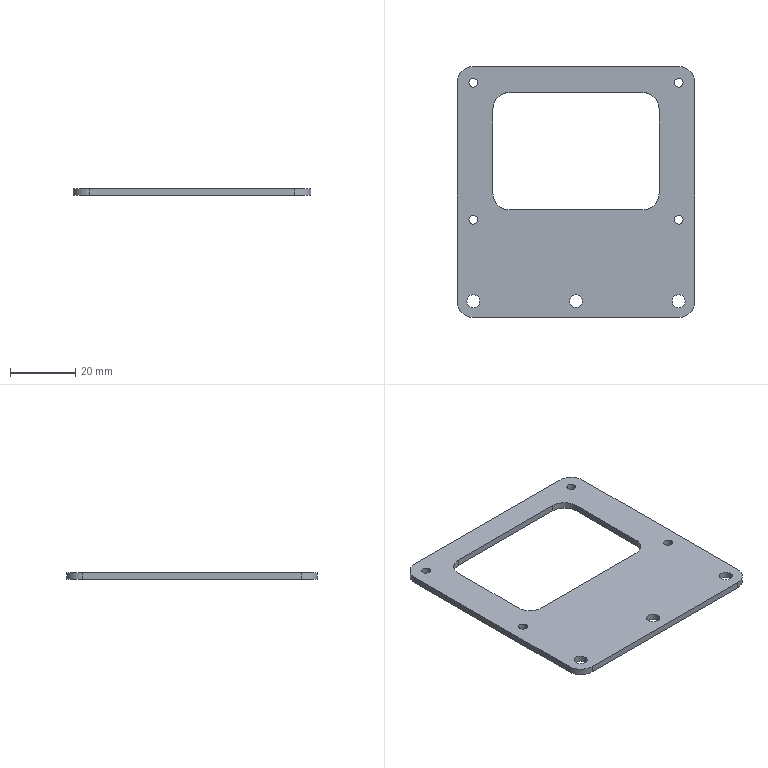Part | SolidWorks | features BaseBody 1 | 1 solid | 32 faces | box 73 x 77 x 2 mm | volume 7449 mm3 | cylinder 22 | plane 10 | commonest cylinder face diameters 2.7 x8 10 x8 4 x6
STEP:
#1=CARTESIAN_POINT('',(-29.5,-46.,2.));
#2=VERTEX_POINT('',#1);
#3=CARTESIAN_POINT('',(-33.5,-46.,2.));
#4=VERTEX_POINT('',#3);
#5=CARTESIAN_POINT('',(-31.5,-46.,2.));
#6=DIRECTION('',(0.,0.,-1.));
#7=DIRECTION('',(-1.,0.,0.));
#8=AXIS2_PLACEMENT_3D('',#5,#6,#7);
#9=CIRCLE('',#8,2.);
#10=EDGE_CURVE('',#2,#4,#9,.T.);
#11=ORIENTED_EDGE('',*,*,#10,.F.);
#12=CARTESIAN_POINT('',(-29.5,-46.,0.));
#13=VERTEX_POINT('',#12);
#14=CARTESIAN_POINT('',(-29.5,-46.,2.));
#15=DIRECTION('',(0.,0.,-1.));
#16=VECTOR('',#15,1000.);
#17=LINE('',#14,#16);
#18=EDGE_CURVE('',#2,#13,#17,.T.);
#19=ORIENTED_EDGE('',*,*,#18,.T.);
#20=CARTESIAN_POINT('',(-33.5,-46.,0.));
#21=VERTEX_POINT('',#20);
#22=CARTESIAN_POINT('',(-31.5,-46.,0.));
#23=DIRECTION('',(0.,0.,-1.));
#24=DIRECTION('',(-1.,0.,0.));
#25=AXIS2_PLACEMENT_3D('',#22,#23,#24);
#26=CIRCLE('',#25,2.);
#27=EDGE_CURVE('',#13,#21,#26,.T.);
#28=ORIENTED_EDGE('',*,*,#27,.T.);
#29=CARTESIAN_POINT('',(-33.5,-46.,2.));
#30=DIRECTION('',(0.,0.,-1.));
#31=VECTOR('',#30,1000.);
#32=LINE('',#29,#31);
#33=EDGE_CURVE('',#4,#21,#32,.T.);
#34=ORIENTED_EDGE('',*,*,#33,.F.);
#35=EDGE_LOOP('',(#11,#19,#28,#34));
#36=FACE_OUTER_BOUND('',#35,.T.);
#37=CARTESIAN_POINT('',(-31.5,-46.,2.));
#38=DIRECTION('',(0.,0.,-1.));
#39=DIRECTION('',(-1.,0.,0.));
#40=AXIS2_PLACEMENT_3D('',#37,#38,#39);
#41=CYLINDRICAL_SURFACE('',#40,2.);
#42=ADVANCED_FACE('',(#36),#41,.F.);
#43=CARTESIAN_POINT('',(33.5,-46.,2.));
#44=VERTEX_POINT('',#43);
#45=CARTESIAN_POINT('',(29.5,-46.,2.));
#46=VERTEX_POINT('',#45);
#47=CARTESIAN_POINT('',(31.5,-46.,2.));
#48=DIRECTION('',(0.,0.,-1.));
#49=DIRECTION('',(-1.,0.,0.));
#50=AXIS2_PLACEMENT_3D('',#47,#48,#49);
#51=CIRCLE('',#50,2.);
#52=EDGE_CURVE('',#44,#46,#51,.T.);
#53=ORIENTED_EDGE('',*,*,#52,.F.);
#54=CARTESIAN_POINT('',(33.5,-46.,0.));
#55=VERTEX_POINT('',#54);
#56=CARTESIAN_POINT('',(33.5,-46.,2.));
#57=DIRECTION('',(0.,0.,-1.));
#58=VECTOR('',#57,1000.);
#59=LINE('',#56,#58);
#60=EDGE_CURVE('',#44,#55,#59,.T.);
#61=ORIENTED_EDGE('',*,*,#60,.T.);
#62=CARTESIAN_POINT('',(29.5,-46.,0.));
#63=VERTEX_POINT('',#62);
#64=CARTESIAN_POINT('',(31.5,-46.,0.));
#65=DIRECTION('',(0.,0.,-1.));
#66=DIRECTION('',(-1.,0.,0.));
#67=AXIS2_PLACEMENT_3D('',#64,#65,#66);
#68=CIRCLE('',#67,2.);
#69=EDGE_CURVE('',#55,#63,#68,.T.);
#70=ORIENTED_EDGE('',*,*,#69,.T.);
#71=CARTESIAN_POINT('',(29.5,-46.,2.));
#72=DIRECTION('',(0.,0.,-1.));
#73=VECTOR('',#72,1000.);
#74=LINE('',#71,#73);
#75=EDGE_CURVE('',#46,#63,#74,.T.);
#76=ORIENTED_EDGE('',*,*,#75,.F.);
#77=EDGE_LOOP('',(#53,#61,#70,#76));
#78=FACE_OUTER_BOUND('',#77,.T.);
#79=CARTESIAN_POINT('',(31.5,-46.,2.));
#80=DIRECTION('',(0.,0.,-1.));
#81=DIRECTION('',(-1.,0.,0.));
#82=AXIS2_PLACEMENT_3D('',#79,#80,#81);
#83=CYLINDRICAL_SURFACE('',#82,2.);
#84=ADVANCED_FACE('',(#78),#83,.F.);
#85=CARTESIAN_POINT('',(2.,-46.,2.));
#86=VERTEX_POINT('',#85);
#87=CARTESIAN_POINT('',(-2.,-46.,2.));
#88=VERTEX_POINT('',#87);
#89=CARTESIAN_POINT('',(0.,-46.,2.));
#90=DIRECTION('',(0.,0.,-1.));
#91=DIRECTION('',(-1.,0.,0.));
#92=AXIS2_PLACEMENT_3D('',#89,#90,#91);
#93=CIRCLE('',#92,2.);
#94=EDGE_CURVE('',#86,#88,#93,.T.);
#95=ORIENTED_EDGE('',*,*,#94,.F.);
#96=CARTESIAN_POINT('',(2.,-46.,0.));
#97=VERTEX_POINT('',#96);
#98=CARTESIAN_POINT('',(2.,-46.,2.));
#99=DIRECTION('',(0.,0.,-1.));
#100=VECTOR('',#99,1000.);
#101=LINE('',#98,#100);
#102=EDGE_CURVE('',#86,#97,#101,.T.);
#103=ORIENTED_EDGE('',*,*,#102,.T.);
#104=CARTESIAN_POINT('',(-2.,-46.,0.));
#105=VERTEX_POINT('',#104);
#106=CARTESIAN_POINT('',(0.,-46.,0.));
#107=DIRECTION('',(0.,0.,-1.));
#108=DIRECTION('',(-1.,0.,0.));
#109=AXIS2_PLACEMENT_3D('',#106,#107,#108);
#110=CIRCLE('',#109,2.);
#111=EDGE_CURVE('',#97,#105,#110,.T.);
#112=ORIENTED_EDGE('',*,*,#111,.T.);
#113=CARTESIAN_POINT('',(-2.,-46.,2.));
#114=DIRECTION('',(0.,0.,-1.));
#115=VECTOR('',#114,1000.);
#116=LINE('',#113,#115);
#117=EDGE_CURVE('',#88,#105,#116,.T.);
#118=ORIENTED_EDGE('',*,*,#117,.F.);
#119=EDGE_LOOP('',(#95,#103,#112,#118));
#120=FACE_OUTER_BOUND('',#119,.T.);
#121=CARTESIAN_POINT('',(0.,-46.,2.));
#122=DIRECTION('',(0.,0.,-1.));
#123=DIRECTION('',(-1.,0.,0.));
#124=AXIS2_PLACEMENT_3D('',#121,#122,#123);
#125=CYLINDRICAL_SURFACE('',#124,2.);
#126=ADVANCED_FACE('',(#120),#125,.F.);
#127=CARTESIAN_POINT('',(-30.15,21.,2.));
#128=VERTEX_POINT('',#127);
#129=CARTESIAN_POINT('',(-32.85,21.,2.));
#130=VERTEX_POINT('',#129);
#131=CARTESIAN_POINT('',(-31.5,21.,2.));
#132=DIRECTION('',(0.,0.,-1.));
#133=DIRECTION('',(-1.,0.,0.));
#134=AXIS2_PLACEMENT_3D('',#131,#132,#133);
#135=CIRCLE('',#134,1.35);
#136=EDGE_CURVE('',#128,#130,#135,.T.);
#137=ORIENTED_EDGE('',*,*,#136,.F.);
#138=CARTESIAN_POINT('',(-30.15,21.,0.));
#139=VERTEX_POINT('',#138);
#140=CARTESIAN_POINT('',(-30.15,21.,2.));
#141=DIRECTION('',(0.,0.,-1.));
#142=VECTOR('',#141,1000.);
#143=LINE('',#140,#142);
#144=EDGE_CURVE('',#128,#139,#143,.T.);
#145=ORIENTED_EDGE('',*,*,#144,.T.);
#146=CARTESIAN_POINT('',(-32.85,21.,0.));
#147=VERTEX_POINT('',#146);
#148=CARTESIAN_POINT('',(-31.5,21.,0.));
#149=DIRECTION('',(0.,0.,-1.));
#150=DIRECTION('',(-1.,0.,0.));
#151=AXIS2_PLACEMENT_3D('',#148,#149,#150);
#152=CIRCLE('',#151,1.35);
#153=EDGE_CURVE('',#139,#147,#152,.T.);
#154=ORIENTED_EDGE('',*,*,#153,.T.);
#155=CARTESIAN_POINT('',(-32.85,21.,2.));
#156=DIRECTION('',(0.,0.,-1.));
#157=VECTOR('',#156,1000.);
#158=LINE('',#155,#157);
#159=EDGE_CURVE('',#130,#147,#158,.T.);
#160=ORIENTED_EDGE('',*,*,#159,.F.);
#161=EDGE_LOOP('',(#137,#145,#154,#160));
#162=FACE_OUTER_BOUND('',#161,.T.);
#163=CARTESIAN_POINT('',(-31.5,21.,2.));
#164=DIRECTION('',(0.,0.,-1.));
#165=DIRECTION('',(-1.,0.,0.));
#166=AXIS2_PLACEMENT_3D('',#163,#164,#165);
#167=CYLINDRICAL_SURFACE('',#166,1.35);
#168=ADVANCED_FACE('',(#162),#167,.F.);
#169=CARTESIAN_POINT('',(-30.15,-21.,2.));
#170=VERTEX_POINT('',#169);
#171=CARTESIAN_POINT('',(-32.85,-21.,2.));
#172=VERTEX_POINT('',#171);
#173=CARTESIAN_POINT('',(-31.5,-21.,2.));
#174=DIRECTION('',(0.,0.,-1.));
#175=DIRECTION('',(-1.,0.,0.));
#176=AXIS2_PLACEMENT_3D('',#173,#174,#175);
#177=CIRCLE('',#176,1.35);
#178=EDGE_CURVE('',#170,#172,#177,.T.);
#179=ORIENTED_EDGE('',*,*,#178,.F.);
#180=CARTESIAN_POINT('',(-30.15,-21.,0.));
#181=VERTEX_POINT('',#180);
#182=CARTESIAN_POINT('',(-30.15,-21.,2.));
#183=DIRECTION('',(0.,0.,-1.));
#184=VECTOR('',#183,1000.);
#185=LINE('',#182,#184);
#186=EDGE_CURVE('',#170,#181,#185,.T.);
#187=ORIENTED_EDGE('',*,*,#186,.T.);
#188=CARTESIAN_POINT('',(-32.85,-21.,0.));
#189=VERTEX_POINT('',#188);
#190=CARTESIAN_POINT('',(-31.5,-21.,0.));
#191=DIRECTION('',(0.,0.,-1.));
#192=DIRECTION('',(-1.,0.,0.));
#193=AXIS2_PLACEMENT_3D('',#190,#191,#192);
#194=CIRCLE('',#193,1.35);
#195=EDGE_CURVE('',#181,#189,#194,.T.);
#196=ORIENTED_EDGE('',*,*,#195,.T.);
#197=CARTESIAN_POINT('',(-32.85,-21.,2.));
#198=DIRECTION('',(0.,0.,-1.));
#199=VECTOR('',#198,1000.);
#200=LINE('',#197,#199);
#201=EDGE_CURVE('',#172,#189,#200,.T.);
#202=ORIENTED_EDGE('',*,*,#201,.F.);
#203=EDGE_LOOP('',(#179,#187,#196,#202));
#204=FACE_OUTER_BOUND('',#203,.T.);
#205=CARTESIAN_POINT('',(-31.5,-21.,2.));
#206=DIRECTION('',(0.,0.,-1.));
#207=DIRECTION('',(-1.,0.,0.));
#208=AXIS2_PLACEMENT_3D('',#205,#206,#207);
#209=CYLINDRICAL_SURFACE('',#208,1.35);
#210=ADVANCED_FACE('',(#204),#209,.F.);
#211=CARTESIAN_POINT('',(32.85,21.,2.));
#212=VERTEX_POINT('',#211);
#213=CARTESIAN_POINT('',(30.15,21.,2.));
#214=VERTEX_POINT('',#213);
#215=CARTESIAN_POINT('',(31.5,21.,2.));
#216=DIRECTION('',(0.,0.,-1.));
#217=DIRECTION('',(-1.,0.,0.));
#218=AXIS2_PLACEMENT_3D('',#215,#216,#217);
#219=CIRCLE('',#218,1.35);
#220=EDGE_CURVE('',#212,#214,#219,.T.);
#221=ORIENTED_EDGE('',*,*,#220,.F.);
#222=CARTESIAN_POINT('',(32.85,21.,0.));
#223=VERTEX_POINT('',#222);
#224=CARTESIAN_POINT('',(32.85,21.,2.));
#225=DIRECTION('',(0.,0.,-1.));
#226=VECTOR('',#225,1000.);
#227=LINE('',#224,#226);
#228=EDGE_CURVE('',#212,#223,#227,.T.);
#229=ORIENTED_EDGE('',*,*,#228,.T.);
#230=CARTESIAN_POINT('',(30.15,21.,0.));
#231=VERTEX_POINT('',#230);
#232=CARTESIAN_POINT('',(31.5,21.,0.));
#233=DIRECTION('',(0.,0.,-1.));
#234=DIRECTION('',(-1.,0.,0.));
#235=AXIS2_PLACEMENT_3D('',#232,#233,#234);
#236=CIRCLE('',#235,1.35);
#237=EDGE_CURVE('',#223,#231,#236,.T.);
#238=ORIENTED_EDGE('',*,*,#237,.T.);
#239=CARTESIAN_POINT('',(30.15,21.,2.));
#240=DIRECTION('',(0.,0.,-1.));
#241=VECTOR('',#240,1000.);
#242=LINE('',#239,#241);
#243=EDGE_CURVE('',#214,#231,#242,.T.);
#244=ORIENTED_EDGE('',*,*,#243,.F.);
#245=EDGE_LOOP('',(#221,#229,#238,#244));
#246=FACE_OUTER_BOUND('',#245,.T.);
#247=CARTESIAN_POINT('',(31.5,21.,2.));
#248=DIRECTION('',(0.,0.,-1.));
#249=DIRECTION('',(-1.,0.,0.));
#250=AXIS2_PLACEMENT_3D('',#247,#248,#249);
#251=CYLINDRICAL_SURFACE('',#250,1.35);
#252=ADVANCED_FACE('',(#246),#251,.F.);
#253=CARTESIAN_POINT('',(32.85,-21.,2.));
#254=VERTEX_POINT('',#253);
#255=CARTESIAN_POINT('',(30.15,-21.,2.));
#256=VERTEX_POINT('',#255);
#257=CARTESIAN_POINT('',(31.5,-21.,2.));
#258=DIRECTION('',(0.,0.,-1.));
#259=DIRECTION('',(-1.,0.,0.));
#260=AXIS2_PLACEMENT_3D('',#257,#258,#259);
#261=CIRCLE('',#260,1.35);
#262=EDGE_CURVE('',#254,#256,#261,.T.);
#263=ORIENTED_EDGE('',*,*,#262,.F.);
#264=CARTESIAN_POINT('',(32.85,-21.,0.));
#265=VERTEX_POINT('',#264);
#266=CARTESIAN_POINT('',(32.85,-21.,2.));
#267=DIRECTION('',(0.,0.,-1.));
#268=VECTOR('',#267,1000.);
#269=LINE('',#266,#268);
#270=EDGE_CURVE('',#254,#265,#269,.T.);
#271=ORIENTED_EDGE('',*,*,#270,.T.);
#272=CARTESIAN_POINT('',(30.15,-21.,0.));
#273=VERTEX_POINT('',#272);
#274=CARTESIAN_POINT('',(31.5,-21.,0.));
#275=DIRECTION('',(0.,0.,-1.));
#276=DIRECTION('',(-1.,0.,0.));
#277=AXIS2_PLACEMENT_3D('',#274,#275,#276);
#278=CIRCLE('',#277,1.35);
#279=EDGE_CURVE('',#265,#273,#278,.T.);
#280=ORIENTED_EDGE('',*,*,#279,.T.);
#281=CARTESIAN_POINT('',(30.15,-21.,2.));
#282=DIRECTION('',(0.,0.,-1.));
#283=VECTOR('',#282,1000.);
#284=LINE('',#281,#283);
#285=EDGE_CURVE('',#256,#273,#284,.T.);
#286=ORIENTED_EDGE('',*,*,#285,.F.);
#287=EDGE_LOOP('',(#263,#271,#280,#286));
#288=FACE_OUTER_BOUND('',#287,.T.);
#289=CARTESIAN_POINT('',(31.5,-21.,2.));
#290=DIRECTION('',(0.,0.,-1.));
#291=DIRECTION('',(-1.,0.,0.));
#292=AXIS2_PLACEMENT_3D('',#289,#290,#291);
#293=CYLINDRICAL_SURFACE('',#292,1.35);
#294=ADVANCED_FACE('',(#288),#293,.F.);
#295=CARTESIAN_POINT('',(-31.5,-46.,0.));
#296=DIRECTION('',(0.,0.,-1.));
#297=DIRECTION('',(-1.,0.,0.));
#298=AXIS2_PLACEMENT_3D('',#295,#296,#297);
#299=CIRCLE('',#298,2.);
#300=EDGE_CURVE('',#21,#13,#299,.T.);
#301=ORIENTED_EDGE('',*,*,#300,.F.);
#302=ORIENTED_EDGE('',*,*,#27,.F.);
#303=EDGE_LOOP('',(#301,#302));
#304=FACE_BOUND('',#303,.T.);
#305=CARTESIAN_POINT('',(31.5,-46.,0.));
#306=DIRECTION('',(0.,0.,-1.));
#307=DIRECTION('',(-1.,0.,0.));
#308=AXIS2_PLACEMENT_3D('',#305,#306,#307);
#309=CIRCLE('',#308,2.);
#310=EDGE_CURVE('',#63,#55,#309,.T.);
#311=ORIENTED_EDGE('',*,*,#310,.F.);
#312=ORIENTED_EDGE('',*,*,#69,.F.);
#313=EDGE_LOOP('',(#311,#312));
#314=FACE_BOUND('',#313,.T.);
#315=CARTESIAN_POINT('',(0.,-46.,0.));
#316=DIRECTION('',(0.,0.,-1.));
#317=DIRECTION('',(-1.,0.,0.));
#318=AXIS2_PLACEMENT_3D('',#315,#316,#317);
#319=CIRCLE('',#318,2.);
#320=EDGE_CURVE('',#105,#97,#319,.T.);
#321=ORIENTED_EDGE('',*,*,#320,.F.);
#322=ORIENTED_EDGE('',*,*,#111,.F.);
#323=EDGE_LOOP('',(#321,#322));
#324=FACE_BOUND('',#323,.T.);
#325=CARTESIAN_POINT('',(-25.5,13.,0.));
#326=VERTEX_POINT('',#325);
#327=CARTESIAN_POINT('',(-20.5,18.,0.));
#328=VERTEX_POINT('',#327);
#329=CARTESIAN_POINT('',(-20.5,13.,0.));
#330=DIRECTION('',(0.,0.,-1.));
#331=DIRECTION('',(-1.,0.,0.));
#332=AXIS2_PLACEMENT_3D('',#329,#330,#331);
#333=CIRCLE('',#332,5.);
#334=EDGE_CURVE('',#326,#328,#333,.T.);
#335=ORIENTED_EDGE('',*,*,#334,.F.);
#336=CARTESIAN_POINT('',(-25.5,-13.,0.));
#337=VERTEX_POINT('',#336);
#338=CARTESIAN_POINT('',(-25.5,0.,0.));
#339=DIRECTION('',(0.,1.,0.));
#340=VECTOR('',#339,1000.);
#341=LINE('',#338,#340);
#342=EDGE_CURVE('',#337,#326,#341,.T.);
#343=ORIENTED_EDGE('',*,*,#342,.F.);
#344=CARTESIAN_POINT('',(-20.5,-18.,0.));
#345=VERTEX_POINT('',#344);
#346=CARTESIAN_POINT('',(-20.5,-13.,0.));
#347=DIRECTION('',(0.,0.,-1.));
#348=DIRECTION('',(1.,0.,0.));
#349=AXIS2_PLACEMENT_3D('',#346,#347,#348);
#350=CIRCLE('',#349,5.);
#351=EDGE_CURVE('',#345,#337,#350,.T.);
#352=ORIENTED_EDGE('',*,*,#351,.F.);
#353=CARTESIAN_POINT('',(20.5,-18.,0.));
#354=VERTEX_POINT('',#353);
#355=CARTESIAN_POINT('',(0.,-18.,0.));
#356=DIRECTION('',(-1.,0.,0.));
#357=VECTOR('',#356,1000.);
#358=LINE('',#355,#357);
#359=EDGE_CURVE('',#354,#345,#358,.T.);
#360=ORIENTED_EDGE('',*,*,#359,.F.);
#361=CARTESIAN_POINT('',(25.5,-13.,0.));
#362=VERTEX_POINT('',#361);
#363=CARTESIAN_POINT('',(20.5,-13.,0.));
#364=DIRECTION('',(0.,0.,-1.));
#365=DIRECTION('',(-1.,0.,0.));
#366=AXIS2_PLACEMENT_3D('',#363,#364,#365);
#367=CIRCLE('',#366,5.);
#368=EDGE_CURVE('',#362,#354,#367,.T.);
#369=ORIENTED_EDGE('',*,*,#368,.F.);
#370=CARTESIAN_POINT('',(25.5,13.,0.));
#371=VERTEX_POINT('',#370);
#372=CARTESIAN_POINT('',(25.5,0.,0.));
#373=DIRECTION('',(0.,-1.,0.));
#374=VECTOR('',#373,1000.);
#375=LINE('',#372,#374);
#376=EDGE_CURVE('',#371,#362,#375,.T.);
#377=ORIENTED_EDGE('',*,*,#376,.F.);
#378=CARTESIAN_POINT('',(20.5,18.,0.));
#379=VERTEX_POINT('',#378);
#380=CARTESIAN_POINT('',(20.5,13.,0.));
#381=DIRECTION('',(0.,0.,-1.));
#382=DIRECTION('',(1.,0.,0.));
#383=AXIS2_PLACEMENT_3D('',#380,#381,#382);
#384=CIRCLE('',#383,5.);
#385=EDGE_CURVE('',#379,#371,#384,.T.);
#386=ORIENTED_EDGE('',*,*,#385,.F.);
#387=CARTESIAN_POINT('',(0.,18.,0.));
#388=DIRECTION('',(1.,0.,0.));
#389=VECTOR('',#388,1000.);
#390=LINE('',#387,#389);
#391=EDGE_CURVE('',#328,#379,#390,.T.);
#392=ORIENTED_EDGE('',*,*,#391,.F.);
#393=EDGE_LOOP('',(#335,#343,#352,#360,#369,#377,#386,#392));
#394=FACE_BOUND('',#393,.T.);
#395=CARTESIAN_POINT('',(-31.5,26.,0.));
#396=VERTEX_POINT('',#395);
#397=CARTESIAN_POINT('',(-36.5,21.,0.));
#398=VERTEX_POINT('',#397);
#399=CARTESIAN_POINT('',(-31.5,21.,0.));
#400=DIRECTION('',(0.,0.,1.));
#401=DIRECTION('',(1.,0.,0.));
#402=AXIS2_PLACEMENT_3D('',#399,#400,#401);
#403=CIRCLE('',#402,5.);
#404=EDGE_CURVE('',#396,#398,#403,.T.);
#405=ORIENTED_EDGE('',*,*,#404,.F.);
#406=CARTESIAN_POINT('',(31.5,26.,0.));
#407=VERTEX_POINT('',#406);
#408=CARTESIAN_POINT('',(0.,26.,0.));
#409=DIRECTION('',(-1.,0.,0.));
#410=VECTOR('',#409,1000.);
#411=LINE('',#408,#410);
#412=EDGE_CURVE('',#407,#396,#411,.T.);
#413=ORIENTED_EDGE('',*,*,#412,.F.);
#414=CARTESIAN_POINT('',(36.5,21.,0.));
#415=VERTEX_POINT('',#414);
#416=CARTESIAN_POINT('',(31.5,21.,0.));
#417=DIRECTION('',(0.,0.,1.));
#418=DIRECTION('',(-1.,0.,0.));
#419=AXIS2_PLACEMENT_3D('',#416,#417,#418);
#420=CIRCLE('',#419,5.);
#421=EDGE_CURVE('',#415,#407,#420,.T.);
#422=ORIENTED_EDGE('',*,*,#421,.F.);
#423=CARTESIAN_POINT('',(36.5,-46.,0.));
#424=VERTEX_POINT('',#423);
#425=CARTESIAN_POINT('',(36.5,0.,0.));
#426=DIRECTION('',(0.,1.,0.));
#427=VECTOR('',#426,1000.);
#428=LINE('',#425,#427);
#429=EDGE_CURVE('',#424,#415,#428,.T.);
#430=ORIENTED_EDGE('',*,*,#429,.F.);
#431=CARTESIAN_POINT('',(31.5,-51.,0.));
#432=VERTEX_POINT('',#431);
#433=CARTESIAN_POINT('',(31.5,-46.,0.));
#434=DIRECTION('',(0.,0.,1.));
#435=DIRECTION('',(1.,0.,0.));
#436=AXIS2_PLACEMENT_3D('',#433,#434,#435);
#437=CIRCLE('',#436,5.);
#438=EDGE_CURVE('',#432,#424,#437,.T.);
#439=ORIENTED_EDGE('',*,*,#438,.F.);
#440=CARTESIAN_POINT('',(-31.5,-51.,0.));
#441=VERTEX_POINT('',#440);
#442=CARTESIAN_POINT('',(0.,-51.,0.));
#443=DIRECTION('',(1.,0.,0.));
#444=VECTOR('',#443,1000.);
#445=LINE('',#442,#444);
#446=EDGE_CURVE('',#441,#432,#445,.T.);
#447=ORIENTED_EDGE('',*,*,#446,.F.);
#448=CARTESIAN_POINT('',(-36.5,-46.,0.));
#449=VERTEX_POINT('',#448);
#450=CARTESIAN_POINT('',(-31.5,-46.,0.));
#451=DIRECTION('',(0.,0.,1.));
#452=DIRECTION('',(-1.,0.,0.));
#453=AXIS2_PLACEMENT_3D('',#450,#451,#452);
#454=CIRCLE('',#453,5.);
#455=EDGE_CURVE('',#449,#441,#454,.T.);
#456=ORIENTED_EDGE('',*,*,#455,.F.);
#457=CARTESIAN_POINT('',(-36.5,0.,0.));
#458=DIRECTION('',(0.,-1.,0.));
#459=VECTOR('',#458,1000.);
#460=LINE('',#457,#459);
#461=EDGE_CURVE('',#398,#449,#460,.T.);
#462=ORIENTED_EDGE('',*,*,#461,.F.);
#463=EDGE_LOOP('',(#405,#413,#422,#430,#439,#447,#456,#462));
#464=FACE_OUTER_BOUND('',#463,.T.);
#465=CARTESIAN_POINT('',(-31.5,21.,0.));
#466=DIRECTION('',(0.,0.,-1.));
#467=DIRECTION('',(-1.,0.,0.));
#468=AXIS2_PLACEMENT_3D('',#465,#466,#467);
#469=CIRCLE('',#468,1.35);
#470=EDGE_CURVE('',#147,#139,#469,.T.);
#471=ORIENTED_EDGE('',*,*,#470,.F.);
#472=ORIENTED_EDGE('',*,*,#153,.F.);
#473=EDGE_LOOP('',(#471,#472));
#474=FACE_BOUND('',#473,.T.);
#475=CARTESIAN_POINT('',(-31.5,-21.,0.));
#476=DIRECTION('',(0.,0.,-1.));
#477=DIRECTION('',(-1.,0.,0.));
#478=AXIS2_PLACEMENT_3D('',#475,#476,#477);
#479=CIRCLE('',#478,1.35);
#480=EDGE_CURVE('',#189,#181,#479,.T.);
#481=ORIENTED_EDGE('',*,*,#480,.F.);
#482=ORIENTED_EDGE('',*,*,#195,.F.);
#483=EDGE_LOOP('',(#481,#482));
#484=FACE_BOUND('',#483,.T.);
#485=CARTESIAN_POINT('',(31.5,21.,0.));
#486=DIRECTION('',(0.,0.,-1.));
#487=DIRECTION('',(-1.,0.,0.));
#488=AXIS2_PLACEMENT_3D('',#485,#486,#487);
#489=CIRCLE('',#488,1.35);
#490=EDGE_CURVE('',#231,#223,#489,.T.);
#491=ORIENTED_EDGE('',*,*,#490,.F.);
#492=ORIENTED_EDGE('',*,*,#237,.F.);
#493=EDGE_LOOP('',(#491,#492));
#494=FACE_BOUND('',#493,.T.);
#495=CARTESIAN_POINT('',(31.5,-21.,0.));
#496=DIRECTION('',(0.,0.,-1.));
#497=DIRECTION('',(-1.,0.,0.));
#498=AXIS2_PLACEMENT_3D('',#495,#496,#497);
#499=CIRCLE('',#498,1.35);
#500=EDGE_CURVE('',#273,#265,#499,.T.);
#501=ORIENTED_EDGE('',*,*,#500,.F.);
#502=ORIENTED_EDGE('',*,*,#279,.F.);
#503=EDGE_LOOP('',(#501,#502));
#504=FACE_BOUND('',#503,.T.);
#505=CARTESIAN_POINT('',(0.,0.,0.));
#506=DIRECTION('',(0.,0.,1.));
#507=DIRECTION('',(1.,0.,0.));
#508=AXIS2_PLACEMENT_3D('',#505,#506,#507);
#509=PLANE('',#508);
#510=ADVANCED_FACE('',(#304,#314,#324,#394,#464,#474,#484,#494,#504),#509,.F.);
#511=ORIENTED_EDGE('',*,*,#18,.F.);
#512=CARTESIAN_POINT('',(-31.5,-46.,2.));
#513=DIRECTION('',(0.,0.,-1.));
#514=DIRECTION('',(-1.,0.,0.));
#515=AXIS2_PLACEMENT_3D('',#512,#513,#514);
#516=CIRCLE('',#515,2.);
#517=EDGE_CURVE('',#4,#2,#516,.T.);
#518=ORIENTED_EDGE('',*,*,#517,.F.);
#519=ORIENTED_EDGE('',*,*,#33,.T.);
#520=ORIENTED_EDGE('',*,*,#300,.T.);
#521=EDGE_LOOP('',(#511,#518,#519,#520));
#522=FACE_OUTER_BOUND('',#521,.T.);
#523=CARTESIAN_POINT('',(-31.5,-46.,2.));
#524=DIRECTION('',(0.,0.,-1.));
#525=DIRECTION('',(-1.,0.,0.));
#526=AXIS2_PLACEMENT_3D('',#523,#524,#525);
#527=CYLINDRICAL_SURFACE('',#526,2.);
#528=ADVANCED_FACE('',(#522),#527,.F.);
#529=ORIENTED_EDGE('',*,*,#60,.F.);
#530=CARTESIAN_POINT('',(31.5,-46.,2.));
#531=DIRECTION('',(0.,0.,-1.));
#532=DIRECTION('',(-1.,0.,0.));
#533=AXIS2_PLACEMENT_3D('',#530,#531,#532);
#534=CIRCLE('',#533,2.);
#535=EDGE_CURVE('',#46,#44,#534,.T.);
#536=ORIENTED_EDGE('',*,*,#535,.F.);
#537=ORIENTED_EDGE('',*,*,#75,.T.);
#538=ORIENTED_EDGE('',*,*,#310,.T.);
#539=EDGE_LOOP('',(#529,#536,#537,#538));
#540=FACE_OUTER_BOUND('',#539,.T.);
#541=CARTESIAN_POINT('',(31.5,-46.,2.));
#542=DIRECTION('',(0.,0.,-1.));
#543=DIRECTION('',(-1.,0.,0.));
#544=AXIS2_PLACEMENT_3D('',#541,#542,#543);
#545=CYLINDRICAL_SURFACE('',#544,2.);
#546=ADVANCED_FACE('',(#540),#545,.F.);
#547=ORIENTED_EDGE('',*,*,#102,.F.);
#548=CARTESIAN_POINT('',(0.,-46.,2.));
#549=DIRECTION('',(0.,0.,-1.));
#550=DIRECTION('',(-1.,0.,0.));
#551=AXIS2_PLACEMENT_3D('',#548,#549,#550);
#552=CIRCLE('',#551,2.);
#553=EDGE_CURVE('',#88,#86,#552,.T.);
#554=ORIENTED_EDGE('',*,*,#553,.F.);
#555=ORIENTED_EDGE('',*,*,#117,.T.);
#556=ORIENTED_EDGE('',*,*,#320,.T.);
#557=EDGE_LOOP('',(#547,#554,#555,#556));
#558=FACE_OUTER_BOUND('',#557,.T.);
#559=CARTESIAN_POINT('',(0.,-46.,2.));
#560=DIRECTION('',(0.,0.,-1.));
#561=DIRECTION('',(-1.,0.,0.));
#562=AXIS2_PLACEMENT_3D('',#559,#560,#561);
#563=CYLINDRICAL_SURFACE('',#562,2.);
#564=ADVANCED_FACE('',(#558),#563,.F.);
#565=CARTESIAN_POINT('',(20.5,18.,2.));
#566=VERTEX_POINT('',#565);
#567=CARTESIAN_POINT('',(20.5,18.,2.));
#568=DIRECTION('',(0.,0.,-1.));
#569=VECTOR('',#568,1000.);
#570=LINE('',#567,#569);
#571=EDGE_CURVE('',#566,#379,#570,.T.);
#572=ORIENTED_EDGE('',*,*,#571,.F.);
#573=CARTESIAN_POINT('',(-20.5,18.,2.));
#574=VERTEX_POINT('',#573);
#575=CARTESIAN_POINT('',(0.,18.,2.));
#576=DIRECTION('',(1.,0.,0.));
#577=VECTOR('',#576,1000.);
#578=LINE('',#575,#577);
#579=EDGE_CURVE('',#574,#566,#578,.T.);
#580=ORIENTED_EDGE('',*,*,#579,.F.);
#581=CARTESIAN_POINT('',(-20.5,18.,2.));
#582=DIRECTION('',(0.,0.,1.));
#583=VECTOR('',#582,1000.);
#584=LINE('',#581,#583);
#585=EDGE_CURVE('',#328,#574,#584,.T.);
#586=ORIENTED_EDGE('',*,*,#585,.F.);
#587=ORIENTED_EDGE('',*,*,#391,.T.);
#588=EDGE_LOOP('',(#572,#580,#586,#587));
#589=FACE_OUTER_BOUND('',#588,.T.);
#590=CARTESIAN_POINT('',(0.,18.,2.));
#591=DIRECTION('',(0.,1.,0.));
#592=DIRECTION('',(0.,0.,1.));
#593=AXIS2_PLACEMENT_3D('',#590,#591,#592);
#594=PLANE('',#593);
#595=ADVANCED_FACE('',(#589),#594,.F.);
#596=CARTESIAN_POINT('',(-25.5,13.,2.));
#597=VERTEX_POINT('',#596);
#598=CARTESIAN_POINT('',(-25.5,13.,2.));
#599=DIRECTION('',(0.,0.,1.));
#600=VECTOR('',#599,1000.);
#601=LINE('',#598,#600);
#602=EDGE_CURVE('',#326,#597,#601,.T.);
#603=ORIENTED_EDGE('',*,*,#602,.F.);
#604=ORIENTED_EDGE('',*,*,#334,.T.);
#605=ORIENTED_EDGE('',*,*,#585,.T.);
#606=CARTESIAN_POINT('',(-20.5,13.,2.));
#607=DIRECTION('',(0.,0.,-1.));
#608=DIRECTION('',(-1.,0.,0.));
#609=AXIS2_PLACEMENT_3D('',#606,#607,#608);
#610=CIRCLE('',#609,5.);
#611=EDGE_CURVE('',#597,#574,#610,.T.);
#612=ORIENTED_EDGE('',*,*,#611,.F.);
#613=EDGE_LOOP('',(#603,#604,#605,#612));
#614=FACE_OUTER_BOUND('',#613,.T.);
#615=CARTESIAN_POINT('',(-20.5,13.,2.));
#616=DIRECTION('',(0.,0.,-1.));
#617=DIRECTION('',(-1.,0.,0.));
#618=AXIS2_PLACEMENT_3D('',#615,#616,#617);
#619=CYLINDRICAL_SURFACE('',#618,5.);
#620=ADVANCED_FACE('',(#614),#619,.F.);
#621=CARTESIAN_POINT('',(-25.5,-13.,2.));
#622=VERTEX_POINT('',#621);
#623=CARTESIAN_POINT('',(-25.5,0.,2.));
#624=DIRECTION('',(0.,-1.,0.));
#625=VECTOR('',#624,1000.);
#626=LINE('',#623,#625);
#627=EDGE_CURVE('',#597,#622,#626,.T.);
#628=ORIENTED_EDGE('',*,*,#627,.T.);
#629=CARTESIAN_POINT('',(-25.5,-13.,2.));
#630=DIRECTION('',(0.,0.,-1.));
#631=VECTOR('',#630,1000.);
#632=LINE('',#629,#631);
#633=EDGE_CURVE('',#622,#337,#632,.T.);
#634=ORIENTED_EDGE('',*,*,#633,.T.);
#635=ORIENTED_EDGE('',*,*,#342,.T.);
#636=ORIENTED_EDGE('',*,*,#602,.T.);
#637=EDGE_LOOP('',(#628,#634,#635,#636));
#638=FACE_OUTER_BOUND('',#637,.T.);
#639=CARTESIAN_POINT('',(-25.5,0.,2.));
#640=DIRECTION('',(1.,0.,0.));
#641=DIRECTION('',(0.,1.,0.));
#642=AXIS2_PLACEMENT_3D('',#639,#640,#641);
#643=PLANE('',#642);
#644=ADVANCED_FACE('',(#638),#643,.T.);
#645=CARTESIAN_POINT('',(-20.5,-18.,2.));
#646=VERTEX_POINT('',#645);
#647=CARTESIAN_POINT('',(-20.5,-18.,2.));
#648=DIRECTION('',(0.,0.,1.));
#649=VECTOR('',#648,1000.);
#650=LINE('',#647,#649);
#651=EDGE_CURVE('',#345,#646,#650,.T.);
#652=ORIENTED_EDGE('',*,*,#651,.F.);
#653=ORIENTED_EDGE('',*,*,#351,.T.);
#654=ORIENTED_EDGE('',*,*,#633,.F.);
#655=CARTESIAN_POINT('',(-20.5,-13.,2.));
#656=DIRECTION('',(0.,0.,-1.));
#657=DIRECTION('',(1.,0.,0.));
#658=AXIS2_PLACEMENT_3D('',#655,#656,#657);
#659=CIRCLE('',#658,5.);
#660=EDGE_CURVE('',#646,#622,#659,.T.);
#661=ORIENTED_EDGE('',*,*,#660,.F.);
#662=EDGE_LOOP('',(#652,#653,#654,#661));
#663=FACE_OUTER_BOUND('',#662,.T.);
#664=CARTESIAN_POINT('',(-20.5,-13.,2.));
#665=DIRECTION('',(0.,0.,1.));
#666=DIRECTION('',(1.,0.,0.));
#667=AXIS2_PLACEMENT_3D('',#664,#665,#666);
#668=CYLINDRICAL_SURFACE('',#667,5.);
#669=ADVANCED_FACE('',(#663),#668,.F.);
#670=CARTESIAN_POINT('',(20.5,-18.,2.));
#671=VERTEX_POINT('',#670);
#672=CARTESIAN_POINT('',(0.,-18.,2.));
#673=DIRECTION('',(1.,0.,0.));
#674=VECTOR('',#673,1000.);
#675=LINE('',#672,#674);
#676=EDGE_CURVE('',#646,#671,#675,.T.);
#677=ORIENTED_EDGE('',*,*,#676,.T.);
#678=CARTESIAN_POINT('',(20.5,-18.,2.));
#679=DIRECTION('',(0.,0.,-1.));
#680=VECTOR('',#679,1000.);
#681=LINE('',#678,#680);
#682=EDGE_CURVE('',#671,#354,#681,.T.);
#683=ORIENTED_EDGE('',*,*,#682,.T.);
#684=ORIENTED_EDGE('',*,*,#359,.T.);
#685=ORIENTED_EDGE('',*,*,#651,.T.);
#686=EDGE_LOOP('',(#677,#683,#684,#685));
#687=FACE_OUTER_BOUND('',#686,.T.);
#688=CARTESIAN_POINT('',(0.,-18.,2.));
#689=DIRECTION('',(0.,1.,0.));
#690=DIRECTION('',(0.,0.,1.));
#691=AXIS2_PLACEMENT_3D('',#688,#689,#690);
#692=PLANE('',#691);
#693=ADVANCED_FACE('',(#687),#692,.T.);
#694=CARTESIAN_POINT('',(25.5,-13.,2.));
#695=VERTEX_POINT('',#694);
#696=CARTESIAN_POINT('',(25.5,-13.,2.));
#697=DIRECTION('',(0.,0.,1.));
#698=VECTOR('',#697,1000.);
#699=LINE('',#696,#698);
#700=EDGE_CURVE('',#362,#695,#699,.T.);
#701=ORIENTED_EDGE('',*,*,#700,.F.);
#702=ORIENTED_EDGE('',*,*,#368,.T.);
#703=ORIENTED_EDGE('',*,*,#682,.F.);
#704=CARTESIAN_POINT('',(20.5,-13.,2.));
#705=DIRECTION('',(0.,0.,-1.));
#706=DIRECTION('',(-1.,0.,0.));
#707=AXIS2_PLACEMENT_3D('',#704,#705,#706);
#708=CIRCLE('',#707,5.);
#709=EDGE_CURVE('',#695,#671,#708,.T.);
#710=ORIENTED_EDGE('',*,*,#709,.F.);
#711=EDGE_LOOP('',(#701,#702,#703,#710));
#712=FACE_OUTER_BOUND('',#711,.T.);
#713=CARTESIAN_POINT('',(20.5,-13.,2.));
#714=DIRECTION('',(0.,0.,-1.));
#715=DIRECTION('',(-1.,0.,0.));
#716=AXIS2_PLACEMENT_3D('',#713,#714,#715);
#717=CYLINDRICAL_SURFACE('',#716,5.);
#718=ADVANCED_FACE('',(#712),#717,.F.);
#719=CARTESIAN_POINT('',(25.5,13.,2.));
#720=VERTEX_POINT('',#719);
#721=CARTESIAN_POINT('',(25.5,13.,2.));
#722=DIRECTION('',(0.,0.,1.));
#723=VECTOR('',#722,1000.);
#724=LINE('',#721,#723);
#725=EDGE_CURVE('',#371,#720,#724,.T.);
#726=ORIENTED_EDGE('',*,*,#725,.F.);
#727=ORIENTED_EDGE('',*,*,#376,.T.);
#728=ORIENTED_EDGE('',*,*,#700,.T.);
#729=CARTESIAN_POINT('',(25.5,0.,2.));
#730=DIRECTION('',(0.,-1.,0.));
#731=VECTOR('',#730,1000.);
#732=LINE('',#729,#731);
#733=EDGE_CURVE('',#720,#695,#732,.T.);
#734=ORIENTED_EDGE('',*,*,#733,.F.);
#735=EDGE_LOOP('',(#726,#727,#728,#734));
#736=FACE_OUTER_BOUND('',#735,.T.);
#737=CARTESIAN_POINT('',(25.5,0.,2.));
#738=DIRECTION('',(1.,0.,0.));
#739=DIRECTION('',(0.,1.,0.));
#740=AXIS2_PLACEMENT_3D('',#737,#738,#739);
#741=PLANE('',#740);
#742=ADVANCED_FACE('',(#736),#741,.F.);
#743=ORIENTED_EDGE('',*,*,#571,.T.);
#744=ORIENTED_EDGE('',*,*,#385,.T.);
#745=ORIENTED_EDGE('',*,*,#725,.T.);
#746=CARTESIAN_POINT('',(20.5,13.,2.));
#747=DIRECTION('',(0.,0.,-1.));
#748=DIRECTION('',(1.,0.,0.));
#749=AXIS2_PLACEMENT_3D('',#746,#747,#748);
#750=CIRCLE('',#749,5.);
#751=EDGE_CURVE('',#566,#720,#750,.T.);
#752=ORIENTED_EDGE('',*,*,#751,.F.);
#753=EDGE_LOOP('',(#743,#744,#745,#752));
#754=FACE_OUTER_BOUND('',#753,.T.);
#755=CARTESIAN_POINT('',(20.5,13.,2.));
#756=DIRECTION('',(0.,0.,1.));
#757=DIRECTION('',(1.,0.,0.));
#758=AXIS2_PLACEMENT_3D('',#755,#756,#757);
#759=CYLINDRICAL_SURFACE('',#758,5.);
#760=ADVANCED_FACE('',(#754),#759,.F.);
#761=CARTESIAN_POINT('',(-36.5,21.,2.));
#762=VERTEX_POINT('',#761);
#763=CARTESIAN_POINT('',(-36.5,21.,2.));
#764=DIRECTION('',(0.,0.,1.));
#765=VECTOR('',#764,1000.);
#766=LINE('',#763,#765);
#767=EDGE_CURVE('',#398,#762,#766,.T.);
#768=ORIENTED_EDGE('',*,*,#767,.F.);
#769=ORIENTED_EDGE('',*,*,#461,.T.);
#770=CARTESIAN_POINT('',(-36.5,-46.,2.));
#771=VERTEX_POINT('',#770);
#772=CARTESIAN_POINT('',(-36.5,-46.,2.));
#773=DIRECTION('',(0.,0.,-1.));
#774=VECTOR('',#773,1000.);
#775=LINE('',#772,#774);
#776=EDGE_CURVE('',#771,#449,#775,.T.);
#777=ORIENTED_EDGE('',*,*,#776,.F.);
#778=CARTESIAN_POINT('',(-36.5,0.,2.));
#779=DIRECTION('',(0.,-1.,0.));
#780=VECTOR('',#779,1000.);
#781=LINE('',#778,#780);
#782=EDGE_CURVE('',#762,#771,#781,.T.);
#783=ORIENTED_EDGE('',*,*,#782,.F.);
#784=EDGE_LOOP('',(#768,#769,#777,#783));
#785=FACE_OUTER_BOUND('',#784,.T.);
#786=CARTESIAN_POINT('',(-36.5,0.,2.));
#787=DIRECTION('',(1.,0.,0.));
#788=DIRECTION('',(0.,0.,-1.));
#789=AXIS2_PLACEMENT_3D('',#786,#787,#788);
#790=PLANE('',#789);
#791=ADVANCED_FACE('',(#785),#790,.F.);
#792=ORIENTED_EDGE('',*,*,#404,.T.);
#793=ORIENTED_EDGE('',*,*,#767,.T.);
#794=CARTESIAN_POINT('',(-31.5,26.,2.));
#795=VERTEX_POINT('',#794);
#796=CARTESIAN_POINT('',(-31.5,21.,2.));
#797=DIRECTION('',(0.,0.,-1.));
#798=DIRECTION('',(1.,0.,0.));
#799=AXIS2_PLACEMENT_3D('',#796,#797,#798);
#800=CIRCLE('',#799,5.);
#801=EDGE_CURVE('',#762,#795,#800,.T.);
#802=ORIENTED_EDGE('',*,*,#801,.T.);
#803=CARTESIAN_POINT('',(-31.5,26.,2.));
#804=DIRECTION('',(0.,0.,-1.));
#805=VECTOR('',#804,1000.);
#806=LINE('',#803,#805);
#807=EDGE_CURVE('',#795,#396,#806,.T.);
#808=ORIENTED_EDGE('',*,*,#807,.T.);
#809=EDGE_LOOP('',(#792,#793,#802,#808));
#810=FACE_OUTER_BOUND('',#809,.T.);
#811=CARTESIAN_POINT('',(-31.5,21.,2.));
#812=DIRECTION('',(0.,0.,1.));
#813=DIRECTION('',(1.,0.,0.));
#814=AXIS2_PLACEMENT_3D('',#811,#812,#813);
#815=CYLINDRICAL_SURFACE('',#814,5.);
#816=ADVANCED_FACE('',(#810),#815,.T.);
#817=CARTESIAN_POINT('',(31.5,26.,2.));
#818=VERTEX_POINT('',#817);
#819=CARTESIAN_POINT('',(0.,26.,2.));
#820=DIRECTION('',(1.,0.,0.));
#821=VECTOR('',#820,1000.);
#822=LINE('',#819,#821);
#823=EDGE_CURVE('',#795,#818,#822,.T.);
#824=ORIENTED_EDGE('',*,*,#823,.T.);
#825=CARTESIAN_POINT('',(31.5,26.,2.));
#826=DIRECTION('',(0.,0.,-1.));
#827=VECTOR('',#826,1000.);
#828=LINE('',#825,#827);
#829=EDGE_CURVE('',#818,#407,#828,.T.);
#830=ORIENTED_EDGE('',*,*,#829,.T.);
#831=ORIENTED_EDGE('',*,*,#412,.T.);
#832=ORIENTED_EDGE('',*,*,#807,.F.);
#833=EDGE_LOOP('',(#824,#830,#831,#832));
#834=FACE_OUTER_BOUND('',#833,.T.);
#835=CARTESIAN_POINT('',(0.,26.,2.));
#836=DIRECTION('',(0.,1.,0.));
#837=DIRECTION('',(-1.,0.,0.));
#838=AXIS2_PLACEMENT_3D('',#835,#836,#837);
#839=PLANE('',#838);
#840=ADVANCED_FACE('',(#834),#839,.T.);
#841=ORIENTED_EDGE('',*,*,#421,.T.);
#842=ORIENTED_EDGE('',*,*,#829,.F.);
#843=CARTESIAN_POINT('',(36.5,21.,2.));
#844=VERTEX_POINT('',#843);
#845=CARTESIAN_POINT('',(31.5,21.,2.));
#846=DIRECTION('',(0.,0.,-1.));
#847=DIRECTION('',(-1.,0.,0.));
#848=AXIS2_PLACEMENT_3D('',#845,#846,#847);
#849=CIRCLE('',#848,5.);
#850=EDGE_CURVE('',#818,#844,#849,.T.);
#851=ORIENTED_EDGE('',*,*,#850,.T.);
#852=CARTESIAN_POINT('',(36.5,21.,2.));
#853=DIRECTION('',(0.,0.,-1.));
#854=VECTOR('',#853,1000.);
#855=LINE('',#852,#854);
#856=EDGE_CURVE('',#844,#415,#855,.T.);
#857=ORIENTED_EDGE('',*,*,#856,.T.);
#858=EDGE_LOOP('',(#841,#842,#851,#857));
#859=FACE_OUTER_BOUND('',#858,.T.);
#860=CARTESIAN_POINT('',(31.5,21.,2.));
#861=DIRECTION('',(0.,0.,-1.));
#862=DIRECTION('',(-1.,0.,0.));
#863=AXIS2_PLACEMENT_3D('',#860,#861,#862);
#864=CYLINDRICAL_SURFACE('',#863,5.);
#865=ADVANCED_FACE('',(#859),#864,.T.);
#866=CARTESIAN_POINT('',(36.5,-46.,2.));
#867=VERTEX_POINT('',#866);
#868=CARTESIAN_POINT('',(36.5,0.,2.));
#869=DIRECTION('',(0.,-1.,0.));
#870=VECTOR('',#869,1000.);
#871=LINE('',#868,#870);
#872=EDGE_CURVE('',#844,#867,#871,.T.);
#873=ORIENTED_EDGE('',*,*,#872,.T.);
#874=CARTESIAN_POINT('',(36.5,-46.,2.));
#875=DIRECTION('',(0.,0.,-1.));
#876=VECTOR('',#875,1000.);
#877=LINE('',#874,#876);
#878=EDGE_CURVE('',#867,#424,#877,.T.);
#879=ORIENTED_EDGE('',*,*,#878,.T.);
#880=ORIENTED_EDGE('',*,*,#429,.T.);
#881=ORIENTED_EDGE('',*,*,#856,.F.);
#882=EDGE_LOOP('',(#873,#879,#880,#881));
#883=FACE_OUTER_BOUND('',#882,.T.);
#884=CARTESIAN_POINT('',(36.5,0.,2.));
#885=DIRECTION('',(1.,0.,0.));
#886=DIRECTION('',(0.,1.,0.));
#887=AXIS2_PLACEMENT_3D('',#884,#885,#886);
#888=PLANE('',#887);
#889=ADVANCED_FACE('',(#883),#888,.T.);
#890=ORIENTED_EDGE('',*,*,#438,.T.);
#891=ORIENTED_EDGE('',*,*,#878,.F.);
#892=CARTESIAN_POINT('',(31.5,-51.,2.));
#893=VERTEX_POINT('',#892);
#894=CARTESIAN_POINT('',(31.5,-46.,2.));
#895=DIRECTION('',(0.,0.,-1.));
#896=DIRECTION('',(1.,0.,0.));
#897=AXIS2_PLACEMENT_3D('',#894,#895,#896);
#898=CIRCLE('',#897,5.);
#899=EDGE_CURVE('',#867,#893,#898,.T.);
#900=ORIENTED_EDGE('',*,*,#899,.T.);
#901=CARTESIAN_POINT('',(31.5,-51.,2.));
#902=DIRECTION('',(0.,0.,-1.));
#903=VECTOR('',#902,1000.);
#904=LINE('',#901,#903);
#905=EDGE_CURVE('',#893,#432,#904,.T.);
#906=ORIENTED_EDGE('',*,*,#905,.T.);
#907=EDGE_LOOP('',(#890,#891,#900,#906));
#908=FACE_OUTER_BOUND('',#907,.T.);
#909=CARTESIAN_POINT('',(31.5,-46.,2.));
#910=DIRECTION('',(0.,0.,1.));
#911=DIRECTION('',(1.,0.,0.));
#912=AXIS2_PLACEMENT_3D('',#909,#910,#911);
#913=CYLINDRICAL_SURFACE('',#912,5.);
#914=ADVANCED_FACE('',(#908),#913,.T.);
#915=ORIENTED_EDGE('',*,*,#905,.F.);
#916=CARTESIAN_POINT('',(-31.5,-51.,2.));
#917=VERTEX_POINT('',#916);
#918=CARTESIAN_POINT('',(0.,-51.,2.));
#919=DIRECTION('',(1.,0.,0.));
#920=VECTOR('',#919,1000.);
#921=LINE('',#918,#920);
#922=EDGE_CURVE('',#917,#893,#921,.T.);
#923=ORIENTED_EDGE('',*,*,#922,.F.);
#924=CARTESIAN_POINT('',(-31.5,-51.,2.));
#925=DIRECTION('',(0.,0.,1.));
#926=VECTOR('',#925,1000.);
#927=LINE('',#924,#926);
#928=EDGE_CURVE('',#441,#917,#927,.T.);
#929=ORIENTED_EDGE('',*,*,#928,.F.);
#930=ORIENTED_EDGE('',*,*,#446,.T.);
#931=EDGE_LOOP('',(#915,#923,#929,#930));
#932=FACE_OUTER_BOUND('',#931,.T.);
#933=CARTESIAN_POINT('',(0.,-51.,2.));
#934=DIRECTION('',(0.,1.,0.));
#935=DIRECTION('',(0.,0.,1.));
#936=AXIS2_PLACEMENT_3D('',#933,#934,#935);
#937=PLANE('',#936);
#938=ADVANCED_FACE('',(#932),#937,.F.);
#939=ORIENTED_EDGE('',*,*,#455,.T.);
#940=ORIENTED_EDGE('',*,*,#928,.T.);
#941=CARTESIAN_POINT('',(-31.5,-46.,2.));
#942=DIRECTION('',(0.,0.,-1.));
#943=DIRECTION('',(-1.,0.,0.));
#944=AXIS2_PLACEMENT_3D('',#941,#942,#943);
#945=CIRCLE('',#944,5.);
#946=EDGE_CURVE('',#917,#771,#945,.T.);
#947=ORIENTED_EDGE('',*,*,#946,.T.);
#948=ORIENTED_EDGE('',*,*,#776,.T.);
#949=EDGE_LOOP('',(#939,#940,#947,#948));
#950=FACE_OUTER_BOUND('',#949,.T.);
#951=CARTESIAN_POINT('',(-31.5,-46.,2.));
#952=DIRECTION('',(0.,0.,-1.));
#953=DIRECTION('',(-1.,0.,0.));
#954=AXIS2_PLACEMENT_3D('',#951,#952,#953);
#955=CYLINDRICAL_SURFACE('',#954,5.);
#956=ADVANCED_FACE('',(#950),#955,.T.);
#957=ORIENTED_EDGE('',*,*,#144,.F.);
#958=CARTESIAN_POINT('',(-31.5,21.,2.));
#959=DIRECTION('',(0.,0.,-1.));
#960=DIRECTION('',(-1.,0.,0.));
#961=AXIS2_PLACEMENT_3D('',#958,#959,#960);
#962=CIRCLE('',#961,1.35);
#963=EDGE_CURVE('',#130,#128,#962,.T.);
#964=ORIENTED_EDGE('',*,*,#963,.F.);
#965=ORIENTED_EDGE('',*,*,#159,.T.);
#966=ORIENTED_EDGE('',*,*,#470,.T.);
#967=EDGE_LOOP('',(#957,#964,#965,#966));
#968=FACE_OUTER_BOUND('',#967,.T.);
#969=CARTESIAN_POINT('',(-31.5,21.,2.));
#970=DIRECTION('',(0.,0.,-1.));
#971=DIRECTION('',(-1.,0.,0.));
#972=AXIS2_PLACEMENT_3D('',#969,#970,#971);
#973=CYLINDRICAL_SURFACE('',#972,1.35);
#974=ADVANCED_FACE('',(#968),#973,.F.);
#975=ORIENTED_EDGE('',*,*,#186,.F.);
#976=CARTESIAN_POINT('',(-31.5,-21.,2.));
#977=DIRECTION('',(0.,0.,-1.));
#978=DIRECTION('',(-1.,0.,0.));
#979=AXIS2_PLACEMENT_3D('',#976,#977,#978);
#980=CIRCLE('',#979,1.35);
#981=EDGE_CURVE('',#172,#170,#980,.T.);
#982=ORIENTED_EDGE('',*,*,#981,.F.);
#983=ORIENTED_EDGE('',*,*,#201,.T.);
#984=ORIENTED_EDGE('',*,*,#480,.T.);
#985=EDGE_LOOP('',(#975,#982,#983,#984));
#986=FACE_OUTER_BOUND('',#985,.T.);
#987=CARTESIAN_POINT('',(-31.5,-21.,2.));
#988=DIRECTION('',(0.,0.,-1.));
#989=DIRECTION('',(-1.,0.,0.));
#990=AXIS2_PLACEMENT_3D('',#987,#988,#989);
#991=CYLINDRICAL_SURFACE('',#990,1.35);
#992=ADVANCED_FACE('',(#986),#991,.F.);
#993=ORIENTED_EDGE('',*,*,#228,.F.);
#994=CARTESIAN_POINT('',(31.5,21.,2.));
#995=DIRECTION('',(0.,0.,-1.));
#996=DIRECTION('',(-1.,0.,0.));
#997=AXIS2_PLACEMENT_3D('',#994,#995,#996);
#998=CIRCLE('',#997,1.35);
#999=EDGE_CURVE('',#214,#212,#998,.T.);
#1000=ORIENTED_EDGE('',*,*,#999,.F.);
#1001=ORIENTED_EDGE('',*,*,#243,.T.);
#1002=ORIENTED_EDGE('',*,*,#490,.T.);
#1003=EDGE_LOOP('',(#993,#1000,#1001,#1002));
#1004=FACE_OUTER_BOUND('',#1003,.T.);
#1005=CARTESIAN_POINT('',(31.5,21.,2.));
#1006=DIRECTION('',(0.,0.,-1.));
#1007=DIRECTION('',(-1.,0.,0.));
#1008=AXIS2_PLACEMENT_3D('',#1005,#1006,#1007);
#1009=CYLINDRICAL_SURFACE('',#1008,1.35);
#1010=ADVANCED_FACE('',(#1004),#1009,.F.);
#1011=ORIENTED_EDGE('',*,*,#270,.F.);
#1012=CARTESIAN_POINT('',(31.5,-21.,2.));
#1013=DIRECTION('',(0.,0.,-1.));
#1014=DIRECTION('',(-1.,0.,0.));
#1015=AXIS2_PLACEMENT_3D('',#1012,#1013,#1014);
#1016=CIRCLE('',#1015,1.35);
#1017=EDGE_CURVE('',#256,#254,#1016,.T.);
#1018=ORIENTED_EDGE('',*,*,#1017,.F.);
#1019=ORIENTED_EDGE('',*,*,#285,.T.);
#1020=ORIENTED_EDGE('',*,*,#500,.T.);
#1021=EDGE_LOOP('',(#1011,#1018,#1019,#1020));
#1022=FACE_OUTER_BOUND('',#1021,.T.);
#1023=CARTESIAN_POINT('',(31.5,-21.,2.));
#1024=DIRECTION('',(0.,0.,-1.));
#1025=DIRECTION('',(-1.,0.,0.));
#1026=AXIS2_PLACEMENT_3D('',#1023,#1024,#1025);
#1027=CYLINDRICAL_SURFACE('',#1026,1.35);
#1028=ADVANCED_FACE('',(#1022),#1027,.F.);
#1029=ORIENTED_EDGE('',*,*,#517,.T.);
#1030=ORIENTED_EDGE('',*,*,#10,.T.);
#1031=EDGE_LOOP('',(#1029,#1030));
#1032=FACE_BOUND('',#1031,.T.);
#1033=ORIENTED_EDGE('',*,*,#535,.T.);
#1034=ORIENTED_EDGE('',*,*,#52,.T.);
#1035=EDGE_LOOP('',(#1033,#1034));
#1036=FACE_BOUND('',#1035,.T.);
#1037=ORIENTED_EDGE('',*,*,#553,.T.);
#1038=ORIENTED_EDGE('',*,*,#94,.T.);
#1039=EDGE_LOOP('',(#1037,#1038));
#1040=FACE_BOUND('',#1039,.T.);
#1041=ORIENTED_EDGE('',*,*,#676,.F.);
#1042=ORIENTED_EDGE('',*,*,#660,.T.);
#1043=ORIENTED_EDGE('',*,*,#627,.F.);
#1044=ORIENTED_EDGE('',*,*,#611,.T.);
#1045=ORIENTED_EDGE('',*,*,#579,.T.);
#1046=ORIENTED_EDGE('',*,*,#751,.T.);
#1047=ORIENTED_EDGE('',*,*,#733,.T.);
#1048=ORIENTED_EDGE('',*,*,#709,.T.);
#1049=EDGE_LOOP('',(#1041,#1042,#1043,#1044,#1045,#1046,#1047,#1048));
#1050=FACE_BOUND('',#1049,.T.);
#1051=ORIENTED_EDGE('',*,*,#872,.F.);
#1052=ORIENTED_EDGE('',*,*,#850,.F.);
#1053=ORIENTED_EDGE('',*,*,#823,.F.);
#1054=ORIENTED_EDGE('',*,*,#801,.F.);
#1055=ORIENTED_EDGE('',*,*,#782,.T.);
#1056=ORIENTED_EDGE('',*,*,#946,.F.);
#1057=ORIENTED_EDGE('',*,*,#922,.T.);
#1058=ORIENTED_EDGE('',*,*,#899,.F.);
#1059=EDGE_LOOP('',(#1051,#1052,#1053,#1054,#1055,#1056,#1057,#1058));
#1060=FACE_OUTER_BOUND('',#1059,.T.);
#1061=ORIENTED_EDGE('',*,*,#963,.T.);
#1062=ORIENTED_EDGE('',*,*,#136,.T.);
#1063=EDGE_LOOP('',(#1061,#1062));
#1064=FACE_BOUND('',#1063,.T.);
#1065=ORIENTED_EDGE('',*,*,#981,.T.);
#1066=ORIENTED_EDGE('',*,*,#178,.T.);
#1067=EDGE_LOOP('',(#1065,#1066));
#1068=FACE_BOUND('',#1067,.T.);
#1069=ORIENTED_EDGE('',*,*,#999,.T.);
#1070=ORIENTED_EDGE('',*,*,#220,.T.);
#1071=EDGE_LOOP('',(#1069,#1070));
#1072=FACE_BOUND('',#1071,.T.);
#1073=ORIENTED_EDGE('',*,*,#1017,.T.);
#1074=ORIENTED_EDGE('',*,*,#262,.T.);
#1075=EDGE_LOOP('',(#1073,#1074));
#1076=FACE_BOUND('',#1075,.T.);
#1077=CARTESIAN_POINT('',(0.,0.,2.));
#1078=DIRECTION('',(0.,0.,1.));
#1079=DIRECTION('',(1.,0.,0.));
#1080=AXIS2_PLACEMENT_3D('',#1077,#1078,#1079);
#1081=PLANE('',#1080);
#1082=ADVANCED_FACE('',(#1032,#1036,#1040,#1050,#1060,#1064,#1068,#1072,#1076),#1081,.T.);
#1083=CLOSED_SHELL('',(#42,#84,#126,#168,#210,#252,#294,#510,#528,#546,#564,#595,#620,#644,#669,#693,#718,#742,#760,#791,#816,#840,#865,#889,#914,#938,#956,#974,#992,#1010,#1028,#1082));
#1084=MANIFOLD_SOLID_BREP('',#1083);
#1085=CARTESIAN_POINT('',(0.,0.,0.));
#1086=DIRECTION('',(0.,0.,1.));
#1087=DIRECTION('',(1.,0.,0.));
#1088=AXIS2_PLACEMENT_3D('',#1085,#1086,#1087);
#1089=(LENGTH_UNIT()NAMED_UNIT(*)SI_UNIT(.MILLI.,.METRE.));
#1090=UNCERTAINTY_MEASURE_WITH_UNIT(LENGTH_MEASURE(0.00001),#1089,'','');
#1091=(NAMED_UNIT(*)PLANE_ANGLE_UNIT()SI_UNIT($,.RADIAN.));
#1092=(NAMED_UNIT(*)SI_UNIT($,.STERADIAN.)SOLID_ANGLE_UNIT());
#1093=(GEOMETRIC_REPRESENTATION_CONTEXT(3)GLOBAL_UNCERTAINTY_ASSIGNED_CONTEXT((#1090))GLOBAL_UNIT_ASSIGNED_CONTEXT((#1089,#1091,#1092))REPRESENTATION_CONTEXT('',''));
#1094=ADVANCED_BREP_SHAPE_REPRESENTATION('',(#1084,#1088),#1093);